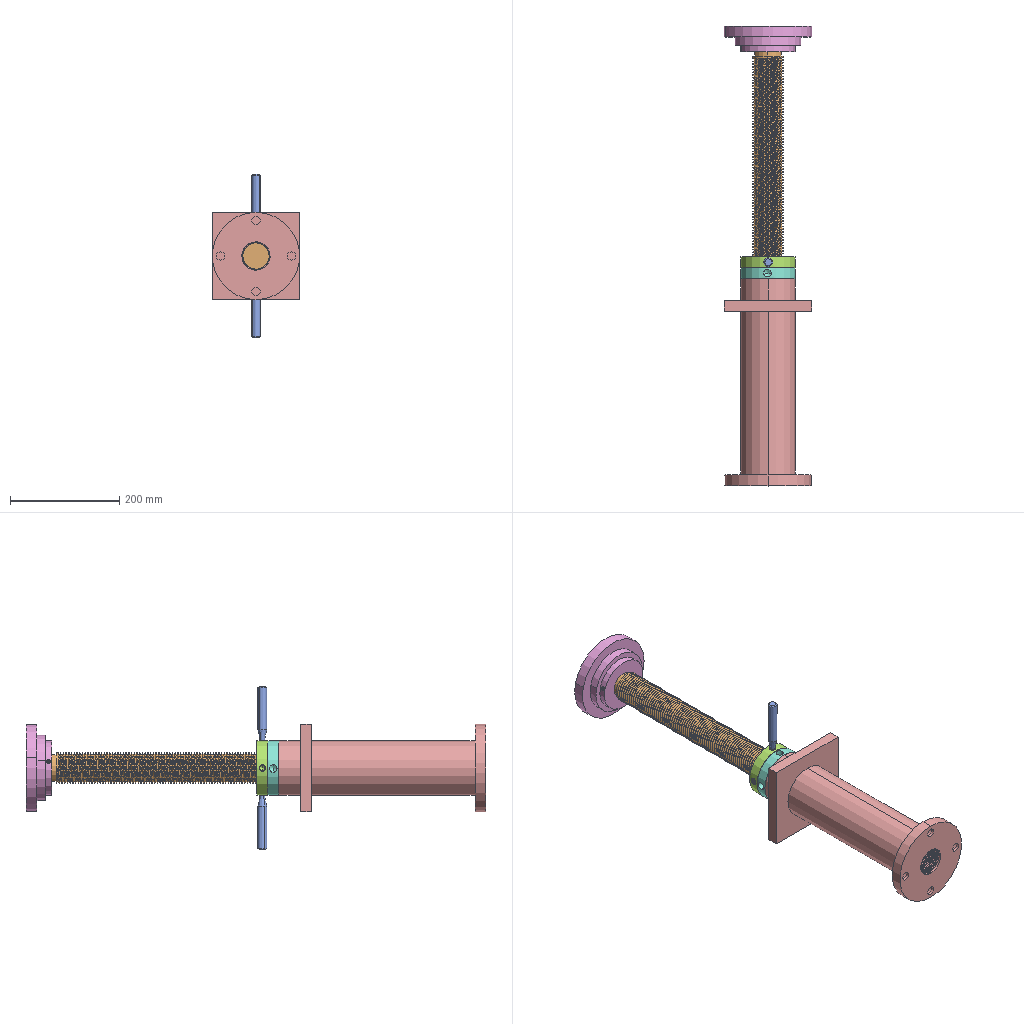Assembly | SolidWorks | 6 different items | 7 placed | box 160 x 843 x 300 mm
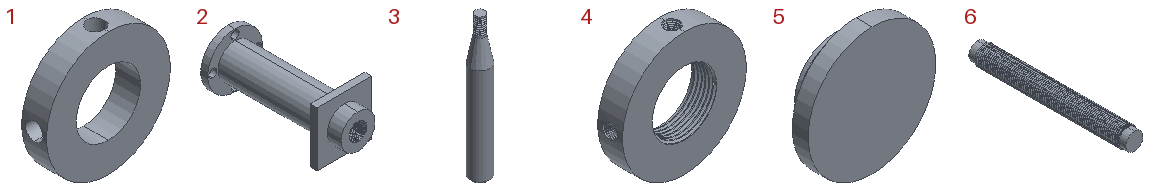Parts list (item | quantity | size | volume | features):
1 | x1 | 100 x 20 x 100 mm | 104092 mm3 | features HoleWzd 2, 3DProfileFeature 1, CirPattern 1, Extrusion 1
2 | x1 | 160 x 380 x 160 mm | 2803979 mm3 | features ICE 3, HoleWzd 2, Extrusion 1, SweepThread 1
3 | x2 | 16 x 16 x 115 mm | 18955 mm3 | features Chamfer 2, Extrusion 1, ICE 1, SweepThread 1
4 | x1 | 100 x 20.124 x 100 mm | 110228 mm3 | features CirPattern 2, HoleWzd 2, SweepThread 2, 3DProfileFeature 1, Extrusion 1
5 | x1 | 160 x 47 x 160 mm | 641630 mm3 | features ICE 4, HoleWzd 2, 3DProfileFeature 1, Extrusion 1, SweepThread 1
6 | x1 | 56 x 450 x 56 mm | 978564 mm3 | features ICE 2, Extrusion 1, SweepThread 1
Mates (type | each side: item.copy, entity, surface, feature):
Concentric | 5.1 face cylinder Boss-Extrude1 | 6.1 face cylinder Boss-Extrude1
Concentric | 5.1 edge | 1.1 face cylinder Boss-Extrude1
Concentric | 4.1 face cylinder Boss-Extrude1 | 1.1 face cylinder Boss-Extrude1
Coincident | 4.1 face plane Boss-Extrude1 | 1.1 face plane Boss-Extrude1
Concentric | 2.1 face cylinder Boss-Extrude1 | 4.1 face cylinder Boss-Extrude1
Coincident | 2.1 face plane Boss-Extrude1 | 1.1 face plane Boss-Extrude1
Coincident | 2.1 plane | assembly plane | 3 times
Concentric | 3.1 face cylinder Boss-Extrude2 | 4.1 face cylinder Ø12.0 (12) Diameter Hole1
Coincident | 5.1 face plane Cut-Extrude1 | 6.1 face plane Boss-Extrude1